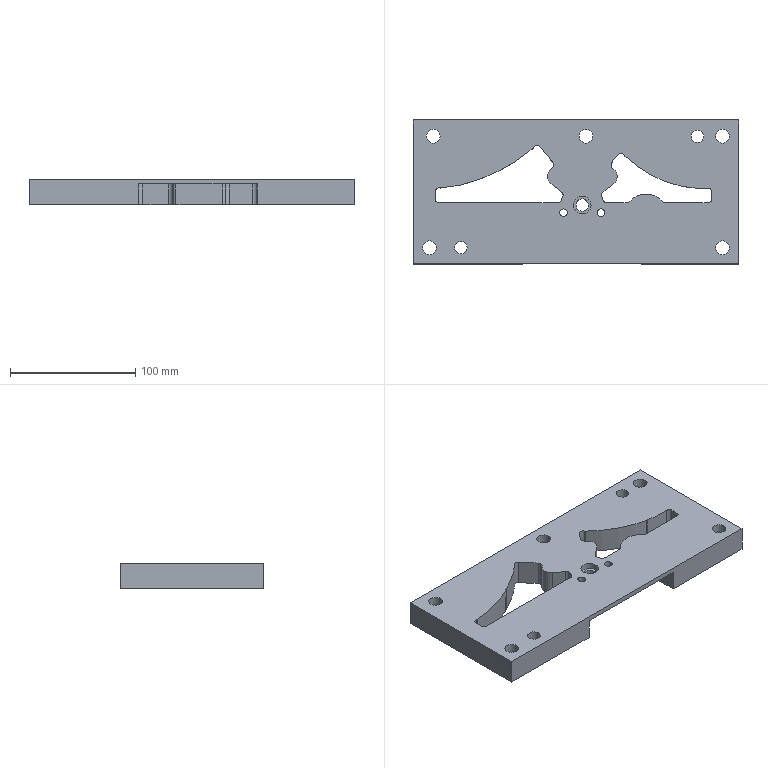Part | STEP file | 406_id3166_x_t | 1 solid | 85 faces | box 260 x 115 x 20 mm | volume 434950 mm3 | cylinder 46 | plane 35 | spline 4 | commonest cylinder face diameters 6 x12 11 x7 7 x6 17 x5 4 x3 10 x3